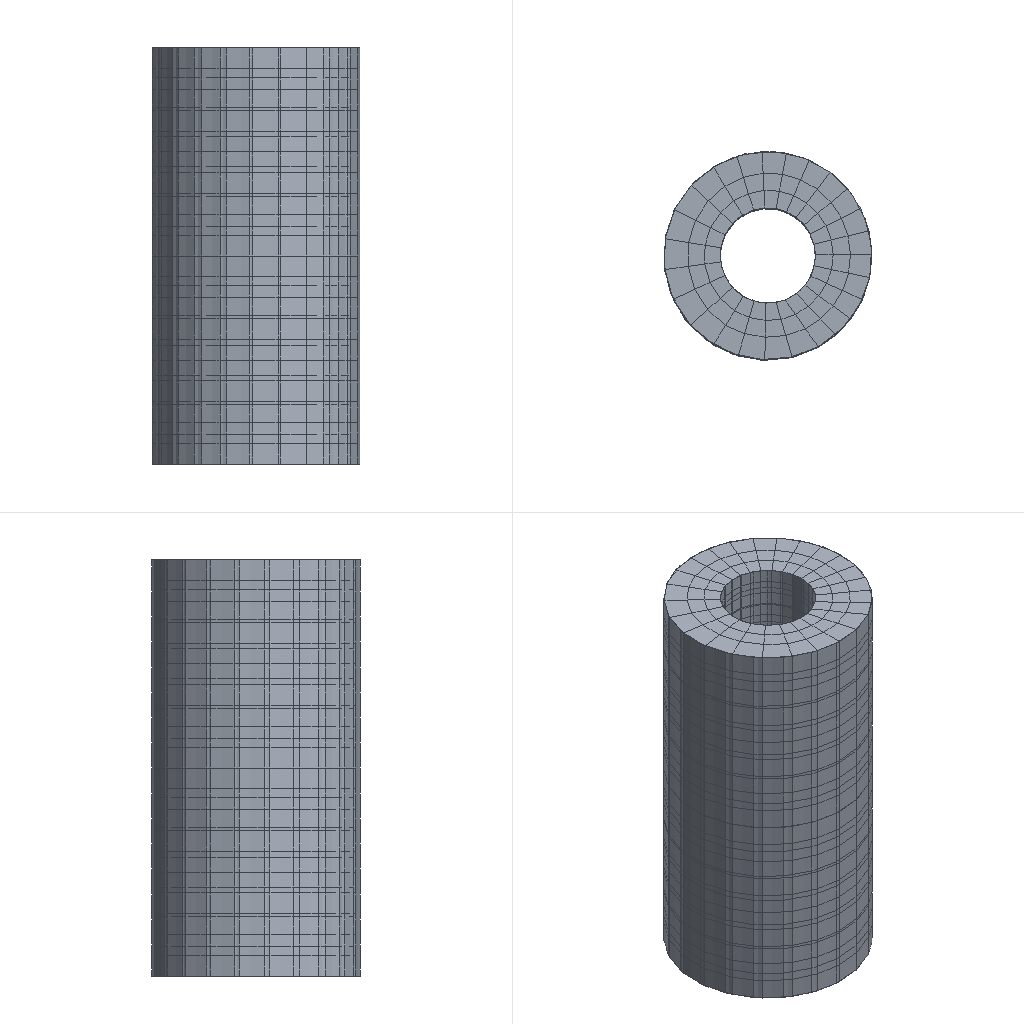Simulation study | abaqus
Set-up summary:
category,name,step,type,value,unit,region
solver,abaqus
solver,version,,,Abaqus/Explicit 2020
units,not stated in the deck,,not stated
analysis,deck,,transient,transient
load_step,Step-1,Step-1,transient
load_step,requested,,,1
mesh,nodes,,,3134
mesh,elements,,,2490
element_type,S4R,,shell,990
element_type,C3D8R,,solid,1500
load,load commands in deck,,count,2
bc,support commands in deck,,count,7
material,CON,,in results
material,FRP,,in results
material,STEEL,,in results
check,setup vs results,,match,"per instance, exact: element labels, types and connectivity; labels of the nodes the elements use; coordinates of those nodes at SINGLE_PRECISION in 3 of 3 instance(s)"
Abaqus input file, long lists of numbers shortened:
*Heading
** Job name: Job-1 Model name: Model-1
** Generated by: Abaqus/CAE 2020
*Preprint, echo=NO, model=NO, history=NO, contact=NO
**
** PARTS
**
*Part, name=cfrp
*Node
      1,   26.02,  -74.387,         305.
      2,   4.384,  -76.093,         305.
** (328 more lines like these left out)
*Element, type=S4R
  1,  22,   1,  23,  44
  2,   1,   2,  24,  23
** (306 more lines like these left out)
*Nset, nset=Set-1, generate
   1,  330,    1
*Elset, elset=Set-1, generate
   1,  308,    1
** Section: cfrp
*Shell Section, elset=Set-1, material=frp
0.17, 5
*End Part
**
*Part, name=con
*Node
      1,  -39.777,  -65.053,           0.
      2,  -18.217,  -29.71,           0.
** (2098 more lines like these left out)
*Element, type=C3D8R
   1,  101,  111,  161,  120,    1,   11,   61,   20
   2,  111,  112,  162,  161,   11,   12,   62,   61
** (1498 more lines like these left out)
*Nset, nset=Set-1, generate
    1,  2100,     1
*Elset, elset=Set-1, generate
    1,  1500,     1
** Section: con
*Solid Section, elset=Set-1, material=con
,
*End Part
**
*Part, name=steel
*Node
      1,    12.25,  -34.723,         305.
      2,   2.347,  -34.153,         305.
** (702 more lines like these left out)
*Element, type=S4R
  1,  22,   1,  23,  44
  2,   1,   2,  24,  23
** (680 more lines like these left out)
*Nset, nset=Set-1, generate
   1,  704,    1
*Elset, elset=Set-1, generate
   1,  682,    1
** Section: steel
*Shell Section, elset=Set-1, material=steel
3.2, 5
*End Part
**
**
** ASSEMBLY
**
*Assembly, name=Assembly
**
*Instance, name=cfrp-1, part=cfrp
   -9.282,           0.,           0.
*End Instance
**
*Instance, name=con-1, part=con
*End Instance
**
*Instance, name=steel-1, part=steel
   -9.282,           0.,           0.
*End Instance
**
*Node
      1, 3.98727281e-07, -2.13394704e-15,         305.
*Nset, nset=Set-1, instance=cfrp-1, generate
 309,  330,    1
*Nset, nset=Set-1, instance=con-1, generate
   1,  100,    1
*Nset, nset=Set-1, instance=steel-1, generate
 683,  704,    1
*Elset, elset=Set-1, instance=cfrp-1, generate
 287,  308,    1
*Elset, elset=Set-1, instance=con-1, generate
  1,  75,   1
*Elset, elset=Set-1, instance=steel-1, generate
 661,  682,    1
*Nset, nset=Set-3
 1,
*Nset, nset=m_Set-2
 1,
*Nset, nset=m_Set-4
 1,
*Nset, nset=s_Set-4, instance=cfrp-1, generate
  1,  22,   1
*Nset, nset=s_Set-4, instance=steel-1, generate
  1,  22,   1
*Nset, nset=s_Set-4
 1,
*Elset, elset=s_Set-4, instance=cfrp-1, generate
  1,  22,   1
*Elset, elset=s_Set-4, instance=steel-1, generate
  1,  22,   1
*Elset, elset=_Surf-7_SPOS, internal, instance=cfrp-1, generate
   1,  308,    1
*Surface, type=ELEMENT, name=Surf-7
_Surf-7_SPOS, SPOS
*Elset, elset=_Surf-8_S6, internal, instance=con-1
    1,    4,    7,   10,   46,   49,   52,   55,   58,   61,   76,   79,   82,   85,  121,  124
  127,  130,  133,  136,  151,  154,  157,  160,  196,  199,  202,  205,  208,  211,  226,  229
** (11 more lines like these left out)
*Elset, elset=_Surf-8_S4, internal, instance=con-1
   15,   18,   21,   24,   27,   30,   33,   36,   39,   42,   45,   66,   69,   72,   75,   90
   93,   96,   99,  102,  105,  108,  111,  114,  117,  120,  141,  144,  147,  150,  165,  168
** (17 more lines like these left out)
*Surface, type=ELEMENT, name=Surf-8
_Surf-8_S6, S6
_Surf-8_S4, S4
*Elset, elset=_Surf-9_SPOS, internal, instance=cfrp-1, generate
   1,  308,    1
*Surface, type=ELEMENT, name=Surf-9
_Surf-9_SPOS, SPOS
*Elset, elset=_m_Surf-2_SNEG, internal, instance=cfrp-1, generate
   1,  308,    1
*Surface, type=ELEMENT, name=m_Surf-2
_m_Surf-2_SNEG, SNEG
*Elset, elset=_m_Surf-4_S4, internal, instance=con-1
    3,    6,    9,   12,   48,   51,   54,   57,   60,   63,   78,   81,   84,   87,  123,  126
  129,  132,  135,  138,  153,  156,  159,  162,  198,  201,  204,  207,  210,  213,  228,  231
** (11 more lines like these left out)
*Elset, elset=_m_Surf-4_S6, internal, instance=con-1
   13,   16,   19,   22,   25,   28,   31,   34,   37,   40,   43,   64,   67,   70,   73,   88
   91,   94,   97,  100,  103,  106,  109,  112,  115,  118,  139,  142,  145,  148,  163,  166
** (17 more lines like these left out)
*Surface, type=ELEMENT, name=m_Surf-4
_m_Surf-4_S4, S4
_m_Surf-4_S6, S6
*Elset, elset=_s_Surf-1_S1, internal, instance=con-1, generate
 1426,  1500,     1
*Surface, type=ELEMENT, name=s_Surf-1
_s_Surf-1_S1, S1
*Elset, elset=_s_Surf-2_S6, internal, instance=con-1
    1,    4,    7,   10,   46,   49,   52,   55,   58,   61,   76,   79,   82,   85,  121,  124
  127,  130,  133,  136,  151,  154,  157,  160,  196,  199,  202,  205,  208,  211,  226,  229
** (11 more lines like these left out)
*Elset, elset=_s_Surf-2_S4, internal, instance=con-1
   15,   18,   21,   24,   27,   30,   33,   36,   39,   42,   45,   66,   69,   72,   75,   90
   93,   96,   99,  102,  105,  108,  111,  114,  117,  120,  141,  144,  147,  150,  165,  168
** (17 more lines like these left out)
*Surface, type=ELEMENT, name=s_Surf-2
_s_Surf-2_S6, S6
_s_Surf-2_S4, S4
*Elset, elset=_s_Surf-4_SPOS, internal, instance=steel-1, generate
   1,  682,    1
*Surface, type=ELEMENT, name=s_Surf-4
_s_Surf-4_SPOS, SPOS
*Elset, elset=_s_Surf-6_S1, internal, instance=con-1, generate
 1426,  1500,     1
*Surface, type=ELEMENT, name=s_Surf-6
_s_Surf-6_S1, S1
*Surface, type=NODE, name=s_Set-4_CNS_, internal
s_Set-4, 1.
** Constraint: Constraint-1
*Coupling, constraint name=Constraint-1, ref node=m_Set-2, surface=s_Surf-6
*Kinematic
** Constraint: Constraint-4
*Coupling, constraint name=Constraint-4, ref node=m_Set-2, surface=s_Set-4_CNS_
*Kinematic
*End Assembly
*Amplitude, name=Amp-1
             0.,              0.,             0.1,              1.
**
** MATERIALS
**
*Material, name=con
*Density
 2.27e-09,
*Elastic
 28394.4, 0.2
*Concrete Damaged Plasticity
30.,     0.1,    1.16, 0.6667,   1e-06
*Concrete Compression Hardening
  10.216,     0.
  14.851, 0.0002
 19.037, 0.0004
 22.773, 0.0006
 26.06, 0.0008
 28.898,  0.001
 31.287, 0.0012
 33.226, 0.0014
 34.716, 0.0016
 35.757, 0.0018
 36.348,  0.002
 36.496, 0.0022
 36.44, 0.0024
 36.315, 0.0026
 36.135, 0.0028
 35.911,  0.003
 35.654, 0.0032
 35.369, 0.0034
 35.064, 0.0036
 34.742, 0.0038
 34.407,  0.004
  34.064, 0.0042
 33.714, 0.0044
 33.36, 0.0046
 33.003, 0.0048
 32.645,  0.005
 31.753, 0.0055
 30.876,  0.006
 30.021, 0.0065
 29.194,  0.007
 28.397, 0.0075
 27.631,  0.008
 26.897, 0.0085
 26.194,  0.009
 25.521, 0.0095
 24.878,   0.01
 24.262, 0.0105
 23.673,  0.011
 23.11, 0.0115
 22.57,  0.012
** (176 more lines like these left out)
*Concrete Tension Stiffening
 3.32,      0.
 1.92,   2e-05
 1.72,   4e-05
 1.53,   6e-05
 1.37,   8e-05
 1.24,  0.0001
 1.13, 0.00011
 1.04, 0.00013
 0.97, 0.00015
  0.9, 0.00016
 0.85, 0.00018
*Concrete Compression Damage
         0.,          0.
         0., 9.81308e-05
         0., 0.0002298
         0., 0.0003774
         0., 0.0005407
         0., 0.0007199
         0., 0.0009147
 0.001545,  0.001117
  0.00498,  0.001321
 0.009911,   0.001527
  0.01603,  0.001735
  0.02309,  0.001944
  0.03089,  0.002154
  0.03926,  0.002365
  0.04808,  0.002576
  0.05724,  0.002788
  0.06665,  0.003
  0.07624,  0.003213
  0.08594,  0.003425
  0.09572,  0.003638
   0.1055,  0.00385
    0.13,   0.004382
   0.154,   0.004913
   0.1774,  0.005443
   0.2001,  0.005972
    0.2219,  0.0065
   0.2429,  0.007027
   0.263,  0.007553
   0.2823,  0.008077
   0.3007,  0.008601
   0.3184,  0.009124
   0.3352,  0.009646
   0.3514,   0.01017
     0.3668,   0.01069
   0.3816,   0.01121
    0.3957,   0.01172
   0.4093,   0.01224
   0.4223,   0.01276
   0.4348,   0.01327
   0.4468,   0.01379
** (171 more lines like these left out)
*Material, name=frp
*Damage Initiation, criterion=HASHIN
1518.,657., 29.,136., 67., 67.
*Density
 2e-09,
*Elastic, type=ENGINEERING CONSTANTS
54000.,54000.,54000.,  0.25,  0.35,  0.35,16000.,24000.
24000.,
*Material, name=steel
*Density
 7.8e-09,
*Elastic
207280., 0.3
*Plastic
 352.7,0.
**
** INTERACTION PROPERTIES
**
*Surface Interaction, name=IntProp-1
*Friction
 0.1,
*Surface Behavior, pressure-overclosure=HARD
**
** INTERACTIONS
**
** Interaction: Int-1
*Contact, op=NEW
*Contact Inclusions, ALL EXTERIOR
*Contact Property Assignment
 ,  , IntProp-1
** ----------------------------------------------------------------
**
** STEP: Step-1
**
*Step, name=Step-1, nlgeom=YES
*Dynamic, Explicit
, 0.1
*Bulk Viscosity
0.06, 1.2
**
** BOUNDARY CONDITIONS
**
** Name: BC-1 Type: 对称/反对称/完全固定
*Boundary
Set-1, ENCASTRE
** Name: BC-2 Type: 位移/转角
*Boundary, amplitude=Amp-1
Set-3, 1, 1
Set-3, 2, 2
Set-3, 3, 3, -30.
Set-3, 4, 4
Set-3, 5, 5
Set-3, 6, 6
**
** LOADS
**
** Name: Load-1   Type: Pressure
*Dsload, amplitude=Amp-1
Surf-9, P, 1.
**
** OUTPUT REQUESTS
**
*Restart, write, number interval=1, time marks=NO
**
** FIELD OUTPUT: F-Output-1
**
*Output, field, number interval=50
*Node Output
CF, RF, RM, RT, U, V
*Element Output, directions=YES
DAMAGEC, DAMAGET, E, LE, MISES, MISESMAX, PE, PEEQ, PEEQMAX, PEEQT, PEMAG, PEQC, S, SDEG, SF, SSAVG
*Contact Output
CDISP, CSTRESS
**
** HISTORY OUTPUT: H-Output-1
**
*Output, history, time interval=5e-05
*Node Output, nset=Set-3
RF3, U3
*End Step
Results summary:
result,step,Step-1,completed,increments=67450 time=0.1/0.1
result,analysis,,,transient
result,last_loadstep,,,1
result,primary field,,,"U, UR"
result,reaction total,,FX,233.494,model units
result,reaction total,,FY,493.457,model units
result,reaction total,,FZ,-375.166,model units